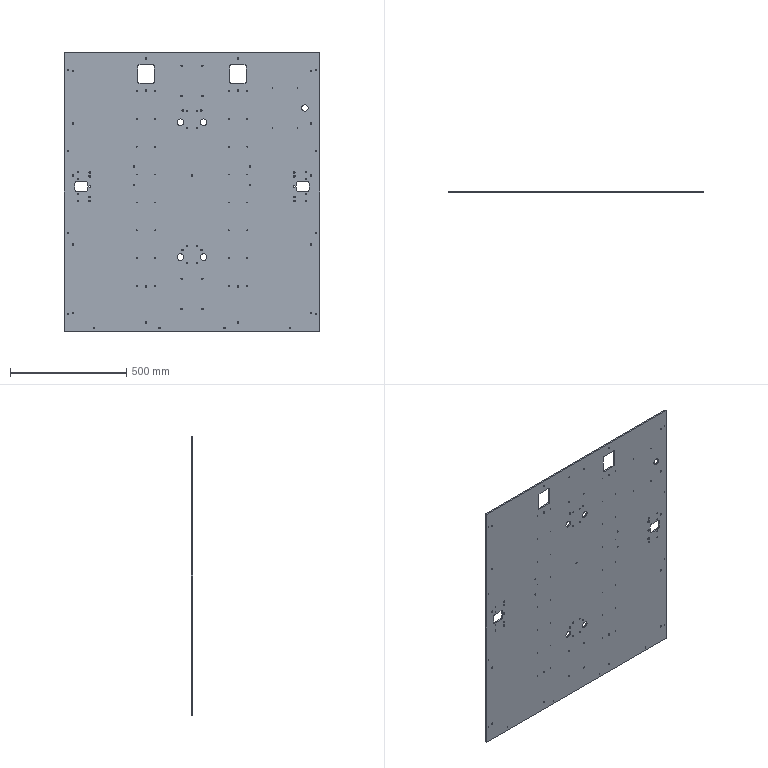Part | SolidWorks | features HoleWzd 12, ICE 3, MirrorPattern 2, Cut 1, Extrusion 1, Fillet 1, LPattern 1 | 1 solid | 270 faces | box 1100 x 6 x 1200 mm | volume 7790456 mm3 | cylinder 248 | plane 22 | commonest cylinder face diameters 3.3 x72 5 x72 6.5 x30 6.8 x16 8 x16 8.5 x12